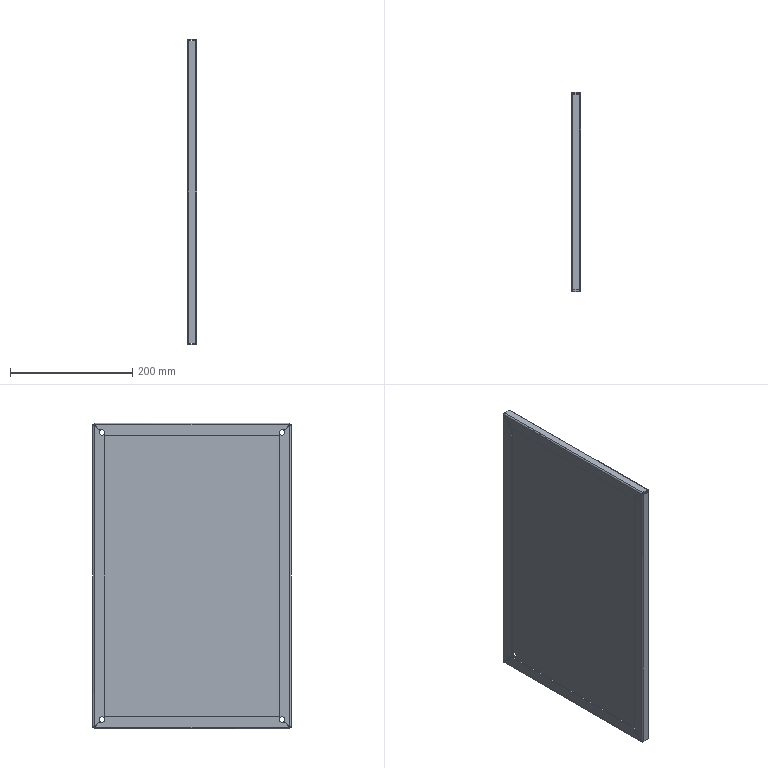Part | SolidWorks | features EdgeFlange 2, FlatPattern 1, ICE 1, SMBaseFlange 1, SheetMetal 1 | 1 solid | 98 faces | box 15 x 325 x 500 mm | volume 418730 mm3 | plane 46 | cylinder 36 | spline 16 | commonest cylinder face diameters 9 x20 0.6 x8 4.6 x8